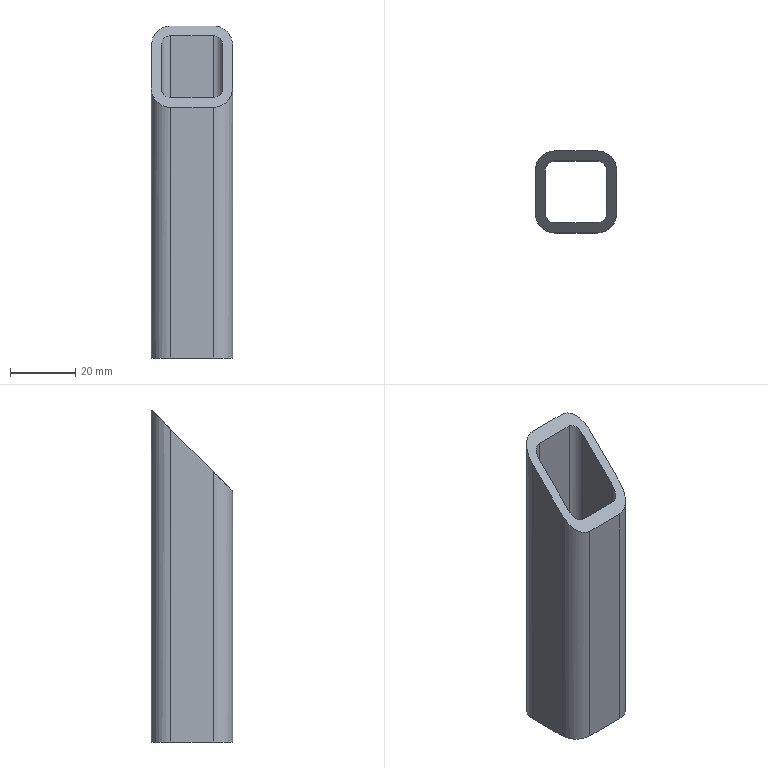Part | STEP file | ISO 10799-2 25x25x3 1784907954397 | 1 solid | 18 faces | box 25 x 25 x 101.928 mm | volume 21536 mm3 | plane 10 | cylinder 8 | commonest cylinder face diameters 6 x4 12 x4
STEP:
#1=CARTESIAN_POINT('',(12.5,6.5,122.172));
#2=VERTEX_POINT('',#1);
#3=CARTESIAN_POINT('',(12.5,-6.5,109.172));
#4=VERTEX_POINT('',#3);
#5=CARTESIAN_POINT('',(12.5,-56.211,59.461));
#6=DIRECTION('',(0.,-0.7071,-0.7071));
#7=VECTOR('',#6,10.);
#8=LINE('',#5,#7);
#9=EDGE_CURVE('',#2,#4,#8,.T.);
#10=ORIENTED_EDGE('',*,*,#9,.F.);
#11=CARTESIAN_POINT('',(6.5,12.5,128.172));
#12=VERTEX_POINT('',#11);
#13=CARTESIAN_POINT('',(6.5,6.5,122.172));
#14=DIRECTION('',(0.,0.7071,-0.7071));
#15=DIRECTION('',(0.,-0.7071,-0.7071));
#16=AXIS2_PLACEMENT_3D('',#13,#14,#15);
#17=ELLIPSE('',#16,8.485,6.);
#18=EDGE_CURVE('',#12,#2,#17,.T.);
#19=ORIENTED_EDGE('',*,*,#18,.F.);
#20=CARTESIAN_POINT('',(-6.5,12.5,128.172));
#21=VERTEX_POINT('',#20);
#22=CARTESIAN_POINT('',(-3.25,12.5,128.172));
#23=DIRECTION('',(1.,0.,0.));
#24=VECTOR('',#23,10.);
#25=LINE('',#22,#24);
#26=EDGE_CURVE('',#21,#12,#25,.T.);
#27=ORIENTED_EDGE('',*,*,#26,.F.);
#28=CARTESIAN_POINT('',(-12.5,6.5,122.172));
#29=VERTEX_POINT('',#28);
#30=CARTESIAN_POINT('',(-6.5,6.5,122.172));
#31=DIRECTION('',(0.,0.7071,-0.7071));
#32=DIRECTION('',(0.,-0.7071,-0.7071));
#33=AXIS2_PLACEMENT_3D('',#30,#31,#32);
#34=ELLIPSE('',#33,8.485,6.);
#35=EDGE_CURVE('',#29,#21,#34,.T.);
#36=ORIENTED_EDGE('',*,*,#35,.F.);
#37=CARTESIAN_POINT('',(-12.5,-6.5,109.172));
#38=VERTEX_POINT('',#37);
#39=CARTESIAN_POINT('',(-12.5,-59.461,56.211));
#40=DIRECTION('',(0.,0.7071,0.7071));
#41=VECTOR('',#40,10.);
#42=LINE('',#39,#41);
#43=EDGE_CURVE('',#38,#29,#42,.T.);
#44=ORIENTED_EDGE('',*,*,#43,.F.);
#45=CARTESIAN_POINT('',(-6.5,-12.5,103.172));
#46=VERTEX_POINT('',#45);
#47=CARTESIAN_POINT('',(-6.5,-6.5,109.172));
#48=DIRECTION('',(0.,0.7071,-0.7071));
#49=DIRECTION('',(0.,0.7071,0.7071));
#50=AXIS2_PLACEMENT_3D('',#47,#48,#49);
#51=ELLIPSE('',#50,8.485,6.);
#52=EDGE_CURVE('',#46,#38,#51,.T.);
#53=ORIENTED_EDGE('',*,*,#52,.F.);
#54=CARTESIAN_POINT('',(6.5,-12.5,103.172));
#55=VERTEX_POINT('',#54);
#56=CARTESIAN_POINT('',(3.25,-12.5,103.172));
#57=DIRECTION('',(-1.,0.,0.));
#58=VECTOR('',#57,10.);
#59=LINE('',#56,#58);
#60=EDGE_CURVE('',#55,#46,#59,.T.);
#61=ORIENTED_EDGE('',*,*,#60,.F.);
#62=CARTESIAN_POINT('',(6.5,-6.5,109.172));
#63=DIRECTION('',(0.,0.7071,-0.7071));
#64=DIRECTION('',(0.,0.7071,0.7071));
#65=AXIS2_PLACEMENT_3D('',#62,#63,#64);
#66=ELLIPSE('',#65,8.485,6.);
#67=EDGE_CURVE('',#4,#55,#66,.T.);
#68=ORIENTED_EDGE('',*,*,#67,.F.);
#69=EDGE_LOOP('',(#10,#19,#27,#36,#44,#53,#61,#68));
#70=FACE_OUTER_BOUND('',#69,.T.);
#71=CARTESIAN_POINT('',(-6.5,-9.5,106.172));
#72=VERTEX_POINT('',#71);
#73=CARTESIAN_POINT('',(6.5,-9.5,106.172));
#74=VERTEX_POINT('',#73);
#75=CARTESIAN_POINT('',(3.25,-9.5,106.172));
#76=DIRECTION('',(1.,0.,0.));
#77=VECTOR('',#76,10.);
#78=LINE('',#75,#77);
#79=EDGE_CURVE('',#72,#74,#78,.T.);
#80=ORIENTED_EDGE('',*,*,#79,.F.);
#81=CARTESIAN_POINT('',(-9.5,-6.5,109.172));
#82=VERTEX_POINT('',#81);
#83=CARTESIAN_POINT('',(-6.5,-6.5,109.172));
#84=DIRECTION('',(0.,-0.7071,0.7071));
#85=DIRECTION('',(0.,0.7071,0.7071));
#86=AXIS2_PLACEMENT_3D('',#83,#84,#85);
#87=ELLIPSE('',#86,4.243,3.);
#88=EDGE_CURVE('',#82,#72,#87,.T.);
#89=ORIENTED_EDGE('',*,*,#88,.F.);
#90=CARTESIAN_POINT('',(-9.5,6.5,122.172));
#91=VERTEX_POINT('',#90);
#92=CARTESIAN_POINT('',(-9.5,-59.461,56.211));
#93=DIRECTION('',(0.,-0.7071,-0.7071));
#94=VECTOR('',#93,10.);
#95=LINE('',#92,#94);
#96=EDGE_CURVE('',#91,#82,#95,.T.);
#97=ORIENTED_EDGE('',*,*,#96,.F.);
#98=CARTESIAN_POINT('',(-6.5,9.5,125.172));
#99=VERTEX_POINT('',#98);
#100=CARTESIAN_POINT('',(-6.5,6.5,122.172));
#101=DIRECTION('',(0.,-0.7071,0.7071));
#102=DIRECTION('',(0.,-0.7071,-0.7071));
#103=AXIS2_PLACEMENT_3D('',#100,#101,#102);
#104=ELLIPSE('',#103,4.243,3.);
#105=EDGE_CURVE('',#99,#91,#104,.T.);
#106=ORIENTED_EDGE('',*,*,#105,.F.);
#107=CARTESIAN_POINT('',(6.5,9.5,125.172));
#108=VERTEX_POINT('',#107);
#109=CARTESIAN_POINT('',(-3.25,9.5,125.172));
#110=DIRECTION('',(-1.,0.,0.));
#111=VECTOR('',#110,10.);
#112=LINE('',#109,#111);
#113=EDGE_CURVE('',#108,#99,#112,.T.);
#114=ORIENTED_EDGE('',*,*,#113,.F.);
#115=CARTESIAN_POINT('',(9.5,6.5,122.172));
#116=VERTEX_POINT('',#115);
#117=CARTESIAN_POINT('',(6.5,6.5,122.172));
#118=DIRECTION('',(0.,-0.7071,0.7071));
#119=DIRECTION('',(0.,-0.7071,-0.7071));
#120=AXIS2_PLACEMENT_3D('',#117,#118,#119);
#121=ELLIPSE('',#120,4.243,3.);
#122=EDGE_CURVE('',#116,#108,#121,.T.);
#123=ORIENTED_EDGE('',*,*,#122,.F.);
#124=CARTESIAN_POINT('',(9.5,-6.5,109.172));
#125=VERTEX_POINT('',#124);
#126=CARTESIAN_POINT('',(9.5,-56.211,59.461));
#127=DIRECTION('',(0.,0.7071,0.7071));
#128=VECTOR('',#127,10.);
#129=LINE('',#126,#128);
#130=EDGE_CURVE('',#125,#116,#129,.T.);
#131=ORIENTED_EDGE('',*,*,#130,.F.);
#132=CARTESIAN_POINT('',(6.5,-6.5,109.172));
#133=DIRECTION('',(0.,-0.7071,0.7071));
#134=DIRECTION('',(0.,0.7071,0.7071));
#135=AXIS2_PLACEMENT_3D('',#132,#133,#134);
#136=ELLIPSE('',#135,4.243,3.);
#137=EDGE_CURVE('',#74,#125,#136,.T.);
#138=ORIENTED_EDGE('',*,*,#137,.F.);
#139=EDGE_LOOP('',(#80,#89,#97,#106,#114,#123,#131,#138));
#140=FACE_BOUND('',#139,.T.);
#141=CARTESIAN_POINT('',(0.,-57.836,57.836));
#142=DIRECTION('',(0.,0.7071,-0.7071));
#143=DIRECTION('',(-1.,0.,0.));
#144=AXIS2_PLACEMENT_3D('',#141,#142,#143);
#145=PLANE('',#144);
#146=ADVANCED_FACE('',(#70,#140),#145,.F.);
#147=ORIENTED_EDGE('',*,*,#113,.T.);
#148=CARTESIAN_POINT('',(-6.5,9.5,26.243));
#149=VERTEX_POINT('',#148);
#150=CARTESIAN_POINT('',(-6.5,9.5,0.));
#151=DIRECTION('',(0.,0.,1.));
#152=VECTOR('',#151,10.);
#153=LINE('',#150,#152);
#154=EDGE_CURVE('',#149,#99,#153,.T.);
#155=ORIENTED_EDGE('',*,*,#154,.F.);
#156=CARTESIAN_POINT('',(6.5,9.5,26.243));
#157=VERTEX_POINT('',#156);
#158=CARTESIAN_POINT('',(-3.25,9.5,26.243));
#159=DIRECTION('',(-1.,0.,0.));
#160=VECTOR('',#159,10.);
#161=LINE('',#158,#160);
#162=EDGE_CURVE('',#157,#149,#161,.T.);
#163=ORIENTED_EDGE('',*,*,#162,.F.);
#164=CARTESIAN_POINT('',(6.5,9.5,0.));
#165=DIRECTION('',(0.,0.,1.));
#166=VECTOR('',#165,10.);
#167=LINE('',#164,#166);
#168=EDGE_CURVE('',#157,#108,#167,.T.);
#169=ORIENTED_EDGE('',*,*,#168,.T.);
#170=EDGE_LOOP('',(#147,#155,#163,#169));
#171=FACE_OUTER_BOUND('',#170,.T.);
#172=CARTESIAN_POINT('',(-6.5,9.5,0.));
#173=DIRECTION('',(0.,1.,0.));
#174=DIRECTION('',(0.,0.,1.));
#175=AXIS2_PLACEMENT_3D('',#172,#173,#174);
#176=PLANE('',#175);
#177=ADVANCED_FACE('',(#171),#176,.F.);
#178=ORIENTED_EDGE('',*,*,#105,.T.);
#179=CARTESIAN_POINT('',(-9.5,6.5,26.243));
#180=VERTEX_POINT('',#179);
#181=CARTESIAN_POINT('',(-9.5,6.5,0.));
#182=DIRECTION('',(0.,0.,1.));
#183=VECTOR('',#182,10.);
#184=LINE('',#181,#183);
#185=EDGE_CURVE('',#180,#91,#184,.T.);
#186=ORIENTED_EDGE('',*,*,#185,.F.);
#187=CARTESIAN_POINT('',(-6.5,6.5,26.243));
#188=DIRECTION('',(0.,0.,1.));
#189=DIRECTION('',(0.,-1.,0.));
#190=AXIS2_PLACEMENT_3D('',#187,#188,#189);
#191=CIRCLE('',#190,3.);
#192=EDGE_CURVE('',#149,#180,#191,.T.);
#193=ORIENTED_EDGE('',*,*,#192,.F.);
#194=ORIENTED_EDGE('',*,*,#154,.T.);
#195=EDGE_LOOP('',(#178,#186,#193,#194));
#196=FACE_OUTER_BOUND('',#195,.T.);
#197=CARTESIAN_POINT('',(-6.5,6.5,0.));
#198=DIRECTION('',(0.,0.,1.));
#199=DIRECTION('',(0.,-1.,0.));
#200=AXIS2_PLACEMENT_3D('',#197,#198,#199);
#201=CYLINDRICAL_SURFACE('',#200,3.);
#202=ADVANCED_FACE('',(#196),#201,.F.);
#203=ORIENTED_EDGE('',*,*,#96,.T.);
#204=CARTESIAN_POINT('',(-9.5,-6.5,26.243));
#205=VERTEX_POINT('',#204);
#206=CARTESIAN_POINT('',(-9.5,-6.5,0.));
#207=DIRECTION('',(0.,0.,1.));
#208=VECTOR('',#207,10.);
#209=LINE('',#206,#208);
#210=EDGE_CURVE('',#205,#82,#209,.T.);
#211=ORIENTED_EDGE('',*,*,#210,.F.);
#212=CARTESIAN_POINT('',(-9.5,-3.25,26.243));
#213=DIRECTION('',(0.,-1.,0.));
#214=VECTOR('',#213,10.);
#215=LINE('',#212,#214);
#216=EDGE_CURVE('',#180,#205,#215,.T.);
#217=ORIENTED_EDGE('',*,*,#216,.F.);
#218=ORIENTED_EDGE('',*,*,#185,.T.);
#219=EDGE_LOOP('',(#203,#211,#217,#218));
#220=FACE_OUTER_BOUND('',#219,.T.);
#221=CARTESIAN_POINT('',(-9.5,-6.5,0.));
#222=DIRECTION('',(-1.,0.,0.));
#223=DIRECTION('',(0.,0.,1.));
#224=AXIS2_PLACEMENT_3D('',#221,#222,#223);
#225=PLANE('',#224);
#226=ADVANCED_FACE('',(#220),#225,.F.);
#227=ORIENTED_EDGE('',*,*,#88,.T.);
#228=CARTESIAN_POINT('',(-6.5,-9.5,26.243));
#229=VERTEX_POINT('',#228);
#230=CARTESIAN_POINT('',(-6.5,-9.5,0.));
#231=DIRECTION('',(0.,0.,1.));
#232=VECTOR('',#231,10.);
#233=LINE('',#230,#232);
#234=EDGE_CURVE('',#229,#72,#233,.T.);
#235=ORIENTED_EDGE('',*,*,#234,.F.);
#236=CARTESIAN_POINT('',(-6.5,-6.5,26.243));
#237=DIRECTION('',(0.,0.,1.));
#238=DIRECTION('',(1.,0.,0.));
#239=AXIS2_PLACEMENT_3D('',#236,#237,#238);
#240=CIRCLE('',#239,3.);
#241=EDGE_CURVE('',#205,#229,#240,.T.);
#242=ORIENTED_EDGE('',*,*,#241,.F.);
#243=ORIENTED_EDGE('',*,*,#210,.T.);
#244=EDGE_LOOP('',(#227,#235,#242,#243));
#245=FACE_OUTER_BOUND('',#244,.T.);
#246=CARTESIAN_POINT('',(-6.5,-6.5,0.));
#247=DIRECTION('',(0.,0.,1.));
#248=DIRECTION('',(1.,0.,0.));
#249=AXIS2_PLACEMENT_3D('',#246,#247,#248);
#250=CYLINDRICAL_SURFACE('',#249,3.);
#251=ADVANCED_FACE('',(#245),#250,.F.);
#252=ORIENTED_EDGE('',*,*,#43,.T.);
#253=CARTESIAN_POINT('',(-12.5,6.5,26.243));
#254=VERTEX_POINT('',#253);
#255=CARTESIAN_POINT('',(-12.5,6.5,0.));
#256=DIRECTION('',(0.,0.,1.));
#257=VECTOR('',#256,10.);
#258=LINE('',#255,#257);
#259=EDGE_CURVE('',#254,#29,#258,.T.);
#260=ORIENTED_EDGE('',*,*,#259,.F.);
#261=CARTESIAN_POINT('',(-12.5,-6.5,26.243));
#262=VERTEX_POINT('',#261);
#263=CARTESIAN_POINT('',(-12.5,-3.25,26.243));
#264=DIRECTION('',(0.,1.,0.));
#265=VECTOR('',#264,10.);
#266=LINE('',#263,#265);
#267=EDGE_CURVE('',#262,#254,#266,.T.);
#268=ORIENTED_EDGE('',*,*,#267,.F.);
#269=CARTESIAN_POINT('',(-12.5,-6.5,0.));
#270=DIRECTION('',(0.,0.,1.));
#271=VECTOR('',#270,10.);
#272=LINE('',#269,#271);
#273=EDGE_CURVE('',#262,#38,#272,.T.);
#274=ORIENTED_EDGE('',*,*,#273,.T.);
#275=EDGE_LOOP('',(#252,#260,#268,#274));
#276=FACE_OUTER_BOUND('',#275,.T.);
#277=CARTESIAN_POINT('',(-12.5,-6.5,0.));
#278=DIRECTION('',(-1.,0.,0.));
#279=DIRECTION('',(0.,0.,1.));
#280=AXIS2_PLACEMENT_3D('',#277,#278,#279);
#281=PLANE('',#280);
#282=ADVANCED_FACE('',(#276),#281,.T.);
#283=ORIENTED_EDGE('',*,*,#35,.T.);
#284=CARTESIAN_POINT('',(-6.5,12.5,26.243));
#285=VERTEX_POINT('',#284);
#286=CARTESIAN_POINT('',(-6.5,12.5,0.));
#287=DIRECTION('',(0.,0.,1.));
#288=VECTOR('',#287,10.);
#289=LINE('',#286,#288);
#290=EDGE_CURVE('',#285,#21,#289,.T.);
#291=ORIENTED_EDGE('',*,*,#290,.F.);
#292=CARTESIAN_POINT('',(-6.5,6.5,26.243));
#293=DIRECTION('',(0.,0.,-1.));
#294=DIRECTION('',(0.,-1.,0.));
#295=AXIS2_PLACEMENT_3D('',#292,#293,#294);
#296=CIRCLE('',#295,6.);
#297=EDGE_CURVE('',#254,#285,#296,.T.);
#298=ORIENTED_EDGE('',*,*,#297,.F.);
#299=ORIENTED_EDGE('',*,*,#259,.T.);
#300=EDGE_LOOP('',(#283,#291,#298,#299));
#301=FACE_OUTER_BOUND('',#300,.T.);
#302=CARTESIAN_POINT('',(-6.5,6.5,0.));
#303=DIRECTION('',(0.,0.,1.));
#304=DIRECTION('',(0.,-1.,0.));
#305=AXIS2_PLACEMENT_3D('',#302,#303,#304);
#306=CYLINDRICAL_SURFACE('',#305,6.);
#307=ADVANCED_FACE('',(#301),#306,.T.);
#308=ORIENTED_EDGE('',*,*,#18,.T.);
#309=CARTESIAN_POINT('',(12.5,6.5,26.243));
#310=VERTEX_POINT('',#309);
#311=CARTESIAN_POINT('',(12.5,6.5,0.));
#312=DIRECTION('',(0.,0.,1.));
#313=VECTOR('',#312,10.);
#314=LINE('',#311,#313);
#315=EDGE_CURVE('',#310,#2,#314,.T.);
#316=ORIENTED_EDGE('',*,*,#315,.F.);
#317=CARTESIAN_POINT('',(6.5,12.5,26.243));
#318=VERTEX_POINT('',#317);
#319=CARTESIAN_POINT('',(6.5,6.5,26.243));
#320=DIRECTION('',(0.,0.,-1.));
#321=DIRECTION('',(-1.,0.,0.));
#322=AXIS2_PLACEMENT_3D('',#319,#320,#321);
#323=CIRCLE('',#322,6.);
#324=EDGE_CURVE('',#318,#310,#323,.T.);
#325=ORIENTED_EDGE('',*,*,#324,.F.);
#326=CARTESIAN_POINT('',(6.5,12.5,0.));
#327=DIRECTION('',(0.,0.,1.));
#328=VECTOR('',#327,10.);
#329=LINE('',#326,#328);
#330=EDGE_CURVE('',#318,#12,#329,.T.);
#331=ORIENTED_EDGE('',*,*,#330,.T.);
#332=EDGE_LOOP('',(#308,#316,#325,#331));
#333=FACE_OUTER_BOUND('',#332,.T.);
#334=CARTESIAN_POINT('',(6.5,6.5,0.));
#335=DIRECTION('',(0.,0.,1.));
#336=DIRECTION('',(-1.,0.,0.));
#337=AXIS2_PLACEMENT_3D('',#334,#335,#336);
#338=CYLINDRICAL_SURFACE('',#337,6.);
#339=ADVANCED_FACE('',(#333),#338,.T.);
#340=ORIENTED_EDGE('',*,*,#79,.T.);
#341=CARTESIAN_POINT('',(6.5,-9.5,26.243));
#342=VERTEX_POINT('',#341);
#343=CARTESIAN_POINT('',(6.5,-9.5,0.));
#344=DIRECTION('',(0.,0.,1.));
#345=VECTOR('',#344,10.);
#346=LINE('',#343,#345);
#347=EDGE_CURVE('',#342,#74,#346,.T.);
#348=ORIENTED_EDGE('',*,*,#347,.F.);
#349=CARTESIAN_POINT('',(3.25,-9.5,26.243));
#350=DIRECTION('',(1.,0.,0.));
#351=VECTOR('',#350,10.);
#352=LINE('',#349,#351);
#353=EDGE_CURVE('',#229,#342,#352,.T.);
#354=ORIENTED_EDGE('',*,*,#353,.F.);
#355=ORIENTED_EDGE('',*,*,#234,.T.);
#356=EDGE_LOOP('',(#340,#348,#354,#355));
#357=FACE_OUTER_BOUND('',#356,.T.);
#358=CARTESIAN_POINT('',(6.5,-9.5,0.));
#359=DIRECTION('',(0.,-1.,0.));
#360=DIRECTION('',(0.,0.,-1.));
#361=AXIS2_PLACEMENT_3D('',#358,#359,#360);
#362=PLANE('',#361);
#363=ADVANCED_FACE('',(#357),#362,.F.);
#364=ORIENTED_EDGE('',*,*,#137,.T.);
#365=CARTESIAN_POINT('',(9.5,-6.5,26.243));
#366=VERTEX_POINT('',#365);
#367=CARTESIAN_POINT('',(9.5,-6.5,0.));
#368=DIRECTION('',(0.,0.,1.));
#369=VECTOR('',#368,10.);
#370=LINE('',#367,#369);
#371=EDGE_CURVE('',#366,#125,#370,.T.);
#372=ORIENTED_EDGE('',*,*,#371,.F.);
#373=CARTESIAN_POINT('',(6.5,-6.5,26.243));
#374=DIRECTION('',(0.,0.,1.));
#375=DIRECTION('',(0.,1.,0.));
#376=AXIS2_PLACEMENT_3D('',#373,#374,#375);
#377=CIRCLE('',#376,3.);
#378=EDGE_CURVE('',#342,#366,#377,.T.);
#379=ORIENTED_EDGE('',*,*,#378,.F.);
#380=ORIENTED_EDGE('',*,*,#347,.T.);
#381=EDGE_LOOP('',(#364,#372,#379,#380));
#382=FACE_OUTER_BOUND('',#381,.T.);
#383=CARTESIAN_POINT('',(6.5,-6.5,0.));
#384=DIRECTION('',(0.,0.,1.));
#385=DIRECTION('',(0.,1.,0.));
#386=AXIS2_PLACEMENT_3D('',#383,#384,#385);
#387=CYLINDRICAL_SURFACE('',#386,3.);
#388=ADVANCED_FACE('',(#382),#387,.F.);
#389=ORIENTED_EDGE('',*,*,#130,.T.);
#390=CARTESIAN_POINT('',(9.5,6.5,26.243));
#391=VERTEX_POINT('',#390);
#392=CARTESIAN_POINT('',(9.5,6.5,0.));
#393=DIRECTION('',(0.,0.,1.));
#394=VECTOR('',#393,10.);
#395=LINE('',#392,#394);
#396=EDGE_CURVE('',#391,#116,#395,.T.);
#397=ORIENTED_EDGE('',*,*,#396,.F.);
#398=CARTESIAN_POINT('',(9.5,3.25,26.243));
#399=DIRECTION('',(0.,1.,0.));
#400=VECTOR('',#399,10.);
#401=LINE('',#398,#400);
#402=EDGE_CURVE('',#366,#391,#401,.T.);
#403=ORIENTED_EDGE('',*,*,#402,.F.);
#404=ORIENTED_EDGE('',*,*,#371,.T.);
#405=EDGE_LOOP('',(#389,#397,#403,#404));
#406=FACE_OUTER_BOUND('',#405,.T.);
#407=CARTESIAN_POINT('',(9.5,6.5,0.));
#408=DIRECTION('',(1.,0.,0.));
#409=DIRECTION('',(0.,0.,-1.));
#410=AXIS2_PLACEMENT_3D('',#407,#408,#409);
#411=PLANE('',#410);
#412=ADVANCED_FACE('',(#406),#411,.F.);
#413=ORIENTED_EDGE('',*,*,#122,.T.);
#414=ORIENTED_EDGE('',*,*,#168,.F.);
#415=CARTESIAN_POINT('',(6.5,6.5,26.243));
#416=DIRECTION('',(0.,0.,1.));
#417=DIRECTION('',(-1.,0.,0.));
#418=AXIS2_PLACEMENT_3D('',#415,#416,#417);
#419=CIRCLE('',#418,3.);
#420=EDGE_CURVE('',#391,#157,#419,.T.);
#421=ORIENTED_EDGE('',*,*,#420,.F.);
#422=ORIENTED_EDGE('',*,*,#396,.T.);
#423=EDGE_LOOP('',(#413,#414,#421,#422));
#424=FACE_OUTER_BOUND('',#423,.T.);
#425=CARTESIAN_POINT('',(6.5,6.5,0.));
#426=DIRECTION('',(0.,0.,1.));
#427=DIRECTION('',(-1.,0.,0.));
#428=AXIS2_PLACEMENT_3D('',#425,#426,#427);
#429=CYLINDRICAL_SURFACE('',#428,3.);
#430=ADVANCED_FACE('',(#424),#429,.F.);
#431=ORIENTED_EDGE('',*,*,#9,.T.);
#432=CARTESIAN_POINT('',(12.5,-6.5,26.243));
#433=VERTEX_POINT('',#432);
#434=CARTESIAN_POINT('',(12.5,-6.5,0.));
#435=DIRECTION('',(0.,0.,1.));
#436=VECTOR('',#435,10.);
#437=LINE('',#434,#436);
#438=EDGE_CURVE('',#433,#4,#437,.T.);
#439=ORIENTED_EDGE('',*,*,#438,.F.);
#440=CARTESIAN_POINT('',(12.5,3.25,26.243));
#441=DIRECTION('',(0.,-1.,0.));
#442=VECTOR('',#441,10.);
#443=LINE('',#440,#442);
#444=EDGE_CURVE('',#310,#433,#443,.T.);
#445=ORIENTED_EDGE('',*,*,#444,.F.);
#446=ORIENTED_EDGE('',*,*,#315,.T.);
#447=EDGE_LOOP('',(#431,#439,#445,#446));
#448=FACE_OUTER_BOUND('',#447,.T.);
#449=CARTESIAN_POINT('',(12.5,6.5,0.));
#450=DIRECTION('',(1.,0.,0.));
#451=DIRECTION('',(0.,0.,-1.));
#452=AXIS2_PLACEMENT_3D('',#449,#450,#451);
#453=PLANE('',#452);
#454=ADVANCED_FACE('',(#448),#453,.T.);
#455=ORIENTED_EDGE('',*,*,#67,.T.);
#456=CARTESIAN_POINT('',(6.5,-12.5,26.243));
#457=VERTEX_POINT('',#456);
#458=CARTESIAN_POINT('',(6.5,-12.5,0.));
#459=DIRECTION('',(0.,0.,1.));
#460=VECTOR('',#459,10.);
#461=LINE('',#458,#460);
#462=EDGE_CURVE('',#457,#55,#461,.T.);
#463=ORIENTED_EDGE('',*,*,#462,.F.);
#464=CARTESIAN_POINT('',(6.5,-6.5,26.243));
#465=DIRECTION('',(0.,0.,-1.));
#466=DIRECTION('',(0.,1.,0.));
#467=AXIS2_PLACEMENT_3D('',#464,#465,#466);
#468=CIRCLE('',#467,6.);
#469=EDGE_CURVE('',#433,#457,#468,.T.);
#470=ORIENTED_EDGE('',*,*,#469,.F.);
#471=ORIENTED_EDGE('',*,*,#438,.T.);
#472=EDGE_LOOP('',(#455,#463,#470,#471));
#473=FACE_OUTER_BOUND('',#472,.T.);
#474=CARTESIAN_POINT('',(6.5,-6.5,0.));
#475=DIRECTION('',(0.,0.,1.));
#476=DIRECTION('',(0.,1.,0.));
#477=AXIS2_PLACEMENT_3D('',#474,#475,#476);
#478=CYLINDRICAL_SURFACE('',#477,6.);
#479=ADVANCED_FACE('',(#473),#478,.T.);
#480=ORIENTED_EDGE('',*,*,#60,.T.);
#481=CARTESIAN_POINT('',(-6.5,-12.5,26.243));
#482=VERTEX_POINT('',#481);
#483=CARTESIAN_POINT('',(-6.5,-12.5,0.));
#484=DIRECTION('',(0.,0.,1.));
#485=VECTOR('',#484,10.);
#486=LINE('',#483,#485);
#487=EDGE_CURVE('',#482,#46,#486,.T.);
#488=ORIENTED_EDGE('',*,*,#487,.F.);
#489=CARTESIAN_POINT('',(3.25,-12.5,26.243));
#490=DIRECTION('',(-1.,0.,0.));
#491=VECTOR('',#490,10.);
#492=LINE('',#489,#491);
#493=EDGE_CURVE('',#457,#482,#492,.T.);
#494=ORIENTED_EDGE('',*,*,#493,.F.);
#495=ORIENTED_EDGE('',*,*,#462,.T.);
#496=EDGE_LOOP('',(#480,#488,#494,#495));
#497=FACE_OUTER_BOUND('',#496,.T.);
#498=CARTESIAN_POINT('',(6.5,-12.5,0.));
#499=DIRECTION('',(0.,-1.,0.));
#500=DIRECTION('',(0.,0.,-1.));
#501=AXIS2_PLACEMENT_3D('',#498,#499,#500);
#502=PLANE('',#501);
#503=ADVANCED_FACE('',(#497),#502,.T.);
#504=ORIENTED_EDGE('',*,*,#52,.T.);
#505=ORIENTED_EDGE('',*,*,#273,.F.);
#506=CARTESIAN_POINT('',(-6.5,-6.5,26.243));
#507=DIRECTION('',(0.,0.,-1.));
#508=DIRECTION('',(1.,0.,0.));
#509=AXIS2_PLACEMENT_3D('',#506,#507,#508);
#510=CIRCLE('',#509,6.);
#511=EDGE_CURVE('',#482,#262,#510,.T.);
#512=ORIENTED_EDGE('',*,*,#511,.F.);
#513=ORIENTED_EDGE('',*,*,#487,.T.);
#514=EDGE_LOOP('',(#504,#505,#512,#513));
#515=FACE_OUTER_BOUND('',#514,.T.);
#516=CARTESIAN_POINT('',(-6.5,-6.5,0.));
#517=DIRECTION('',(0.,0.,1.));
#518=DIRECTION('',(1.,0.,0.));
#519=AXIS2_PLACEMENT_3D('',#516,#517,#518);
#520=CYLINDRICAL_SURFACE('',#519,6.);
#521=ADVANCED_FACE('',(#515),#520,.T.);
#522=ORIENTED_EDGE('',*,*,#26,.T.);
#523=ORIENTED_EDGE('',*,*,#330,.F.);
#524=CARTESIAN_POINT('',(-3.25,12.5,26.243));
#525=DIRECTION('',(1.,0.,0.));
#526=VECTOR('',#525,10.);
#527=LINE('',#524,#526);
#528=EDGE_CURVE('',#285,#318,#527,.T.);
#529=ORIENTED_EDGE('',*,*,#528,.F.);
#530=ORIENTED_EDGE('',*,*,#290,.T.);
#531=EDGE_LOOP('',(#522,#523,#529,#530));
#532=FACE_OUTER_BOUND('',#531,.T.);
#533=CARTESIAN_POINT('',(-6.5,12.5,0.));
#534=DIRECTION('',(0.,1.,0.));
#535=DIRECTION('',(0.,0.,1.));
#536=AXIS2_PLACEMENT_3D('',#533,#534,#535);
#537=PLANE('',#536);
#538=ADVANCED_FACE('',(#532),#537,.T.);
#539=ORIENTED_EDGE('',*,*,#267,.T.);
#540=ORIENTED_EDGE('',*,*,#297,.T.);
#541=ORIENTED_EDGE('',*,*,#528,.T.);
#542=ORIENTED_EDGE('',*,*,#324,.T.);
#543=ORIENTED_EDGE('',*,*,#444,.T.);
#544=ORIENTED_EDGE('',*,*,#469,.T.);
#545=ORIENTED_EDGE('',*,*,#493,.T.);
#546=ORIENTED_EDGE('',*,*,#511,.T.);
#547=EDGE_LOOP('',(#539,#540,#541,#542,#543,#544,#545,#546));
#548=FACE_OUTER_BOUND('',#547,.T.);
#549=ORIENTED_EDGE('',*,*,#162,.T.);
#550=ORIENTED_EDGE('',*,*,#192,.T.);
#551=ORIENTED_EDGE('',*,*,#216,.T.);
#552=ORIENTED_EDGE('',*,*,#241,.T.);
#553=ORIENTED_EDGE('',*,*,#353,.T.);
#554=ORIENTED_EDGE('',*,*,#378,.T.);
#555=ORIENTED_EDGE('',*,*,#402,.T.);
#556=ORIENTED_EDGE('',*,*,#420,.T.);
#557=EDGE_LOOP('',(#549,#550,#551,#552,#553,#554,#555,#556));
#558=FACE_BOUND('',#557,.T.);
#559=CARTESIAN_POINT('',(0.,0.,26.243));
#560=DIRECTION('',(0.,0.,1.));
#561=DIRECTION('',(1.,0.,0.));
#562=AXIS2_PLACEMENT_3D('',#559,#560,#561);
#563=PLANE('',#562);
#564=ADVANCED_FACE('',(#548,#558),#563,.F.);
#565=CLOSED_SHELL('',(#146,#177,#202,#226,#251,#282,#307,#339,#363,#388,#412,#430,#454,#479,#503,#521,#538,#564));
#566=MANIFOLD_SOLID_BREP('',#565);
#567=(LENGTH_UNIT()NAMED_UNIT(*)SI_UNIT(.MILLI.,.METRE.));
#568=UNCERTAINTY_MEASURE_WITH_UNIT(LENGTH_MEASURE(0.01),#567,'','');
#569=(NAMED_UNIT(*)PLANE_ANGLE_UNIT()SI_UNIT($,.RADIAN.));
#570=(NAMED_UNIT(*)SI_UNIT($,.STERADIAN.)SOLID_ANGLE_UNIT());
#571=(GEOMETRIC_REPRESENTATION_CONTEXT(3)GLOBAL_UNCERTAINTY_ASSIGNED_CONTEXT((#568))GLOBAL_UNIT_ASSIGNED_CONTEXT((#567,#569,#570))REPRESENTATION_CONTEXT('',''));
#572=ADVANCED_BREP_SHAPE_REPRESENTATION('',(#566),#571);